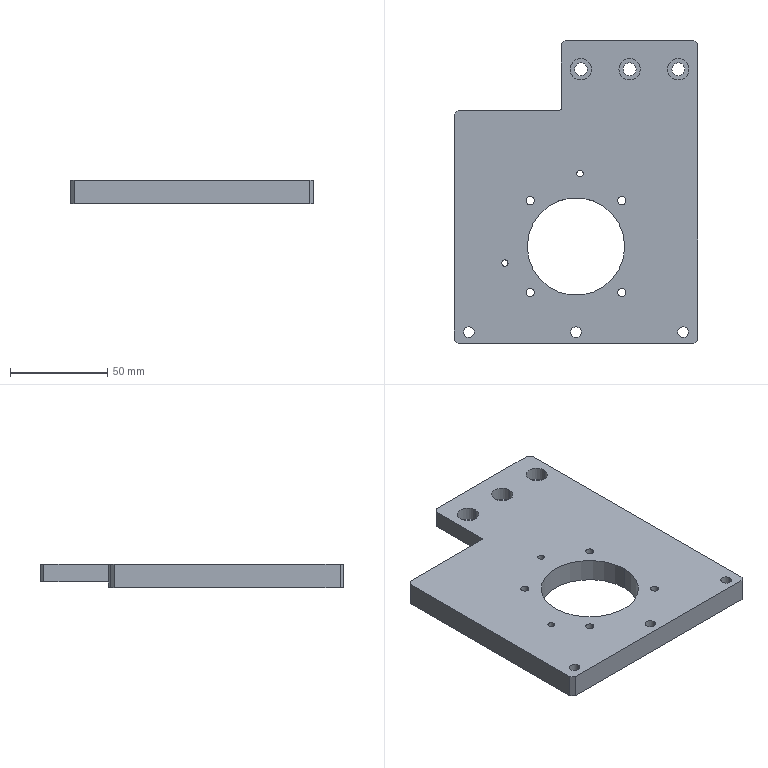Part | SolidWorks | features HoleWzd 4, ICE 3, Chamfer 1, Extrusion 1, Fillet 1 | 1 solid | 60 faces | box 125 x 156 x 12 mm | volume 174396 mm3 | cylinder 39 | plane 21 | commonest cylinder face diameters 4.2 x8 5.5 x6 6.6 x6 10 x6 11 x6 3.3 x4